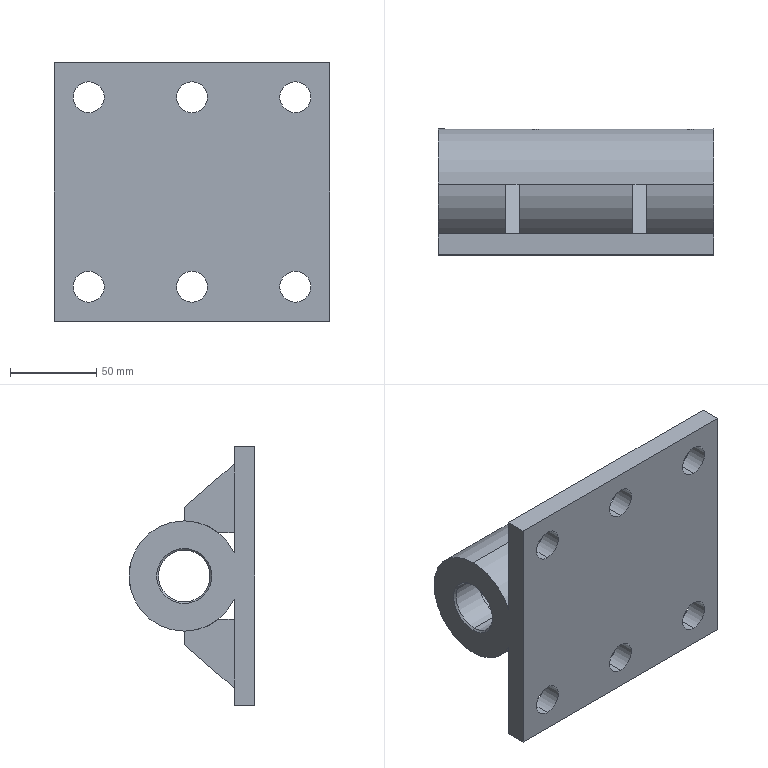Part | SolidWorks | features MirrorStock 1 | 5 solids | 66 faces | box 160 x 73 x 150 mm | volume 566023 mm3 | plane 33 | cylinder 29 | cone 4 | commonest cylinder face diameters 18 x12 64 x7 8.5 x4 30 x2 40 x2 46 x2